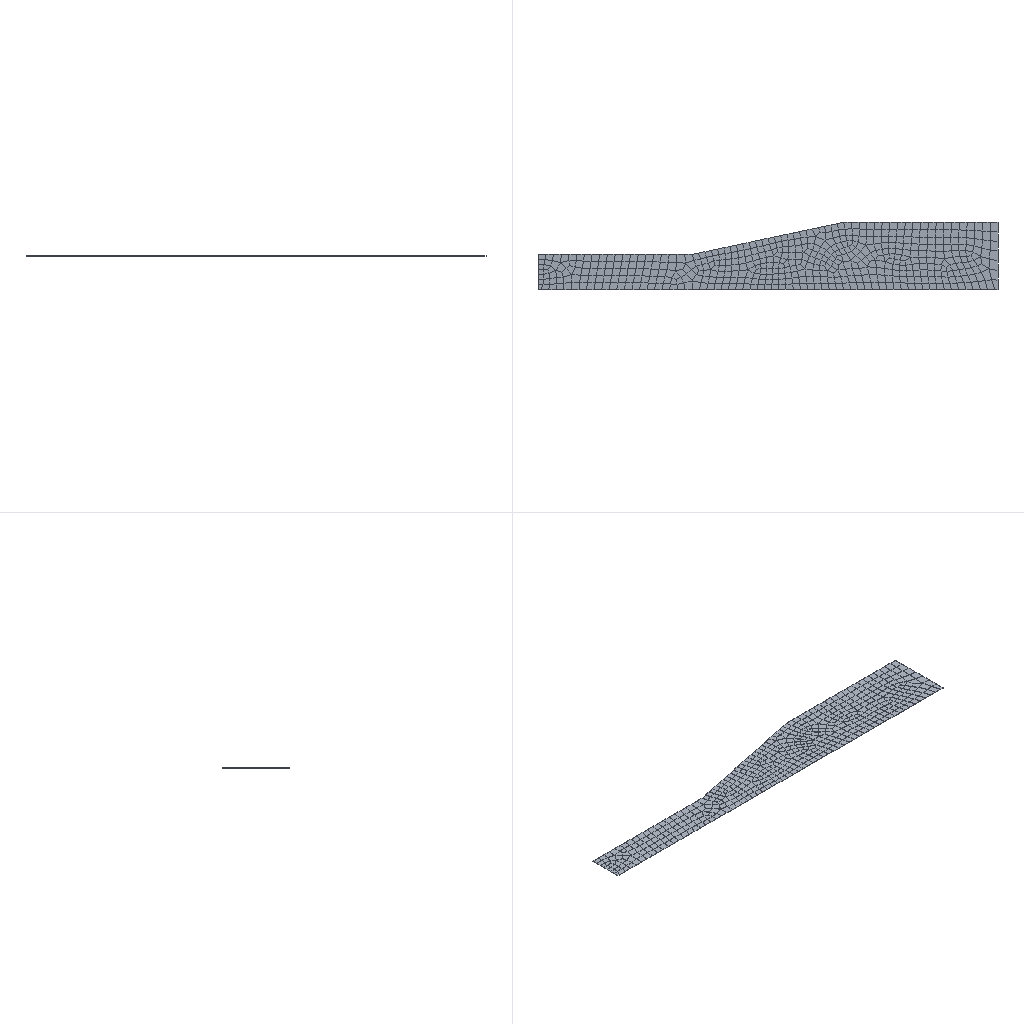Simulation study | abaqus
Set-up summary:
category,name,step,type,value,unit,region
solver,abaqus
solver,version,,,Abaqus/Standard 2020
units,not stated in the deck,,not stated
analysis,deck,,geostatic,geostatic; transient
load_step,geo,geo,geostatic,nlgeom=True
load_step,ear,ear,transient,nlgeom=True
contact,interactions,,,general=0 pairs=0 ties=0
load_step,requested,,,2
mesh,nodes,,,1180
mesh,elements,,,518
element_type,C3D8,,solid,518
load,load commands in deck,,count,2
bc,support commands in deck,,count,7
material,MATERIAL-1,,in results
check,setup vs results,,match,"per instance, exact: element labels, types and connectivity; labels of the nodes the elements use; coordinates of those nodes at SINGLE_PRECISION in 1 of 1 instance(s)"
Results summary:
result,step,,completed,increments=11 time=1.0/1.0
result,step,,partial,increments=1125 time=22.5/22.5
result,analysis,,,transient
result,last_loadstep,,,2
result,analysis steps,,count,2
result,primary field,,,U
result,reaction total,,FX,79739585.562,model units
result,reaction total,,FY,4056211832.875,model units
result,reaction total,,FZ,0.0,model units